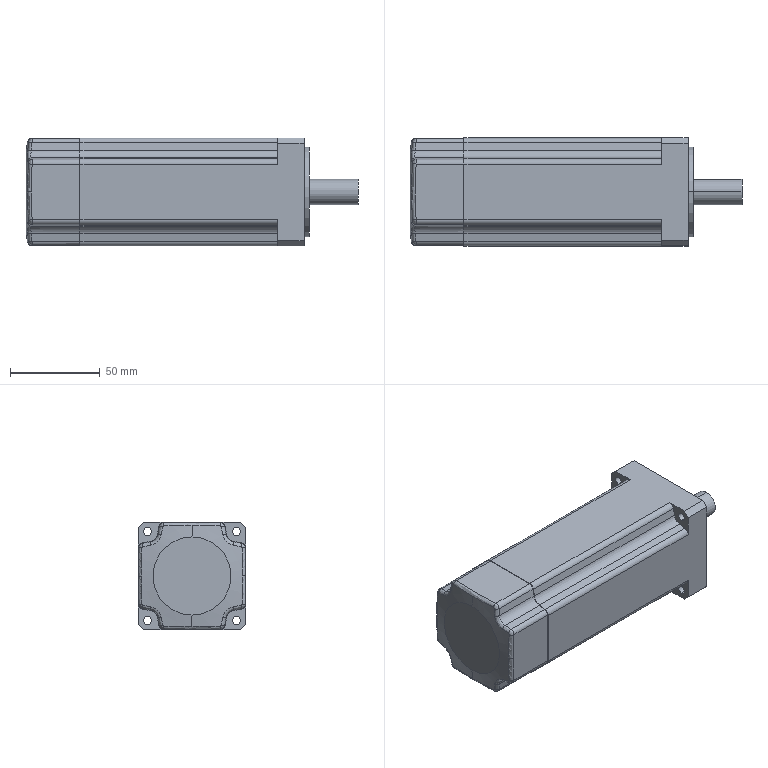Part | STEP file | Panasonic A4 servo motor (400W220V) | 1 solid | 101 faces | box 184.5 x 60 x 60 mm | volume 493168 mm3 | plane 37 | cylinder 36 | spline 26 | cone 2 | commonest cylinder face diameters 4.5 x8 5.4 x8 6 x8 10 x4 10.6 x4 14 x2